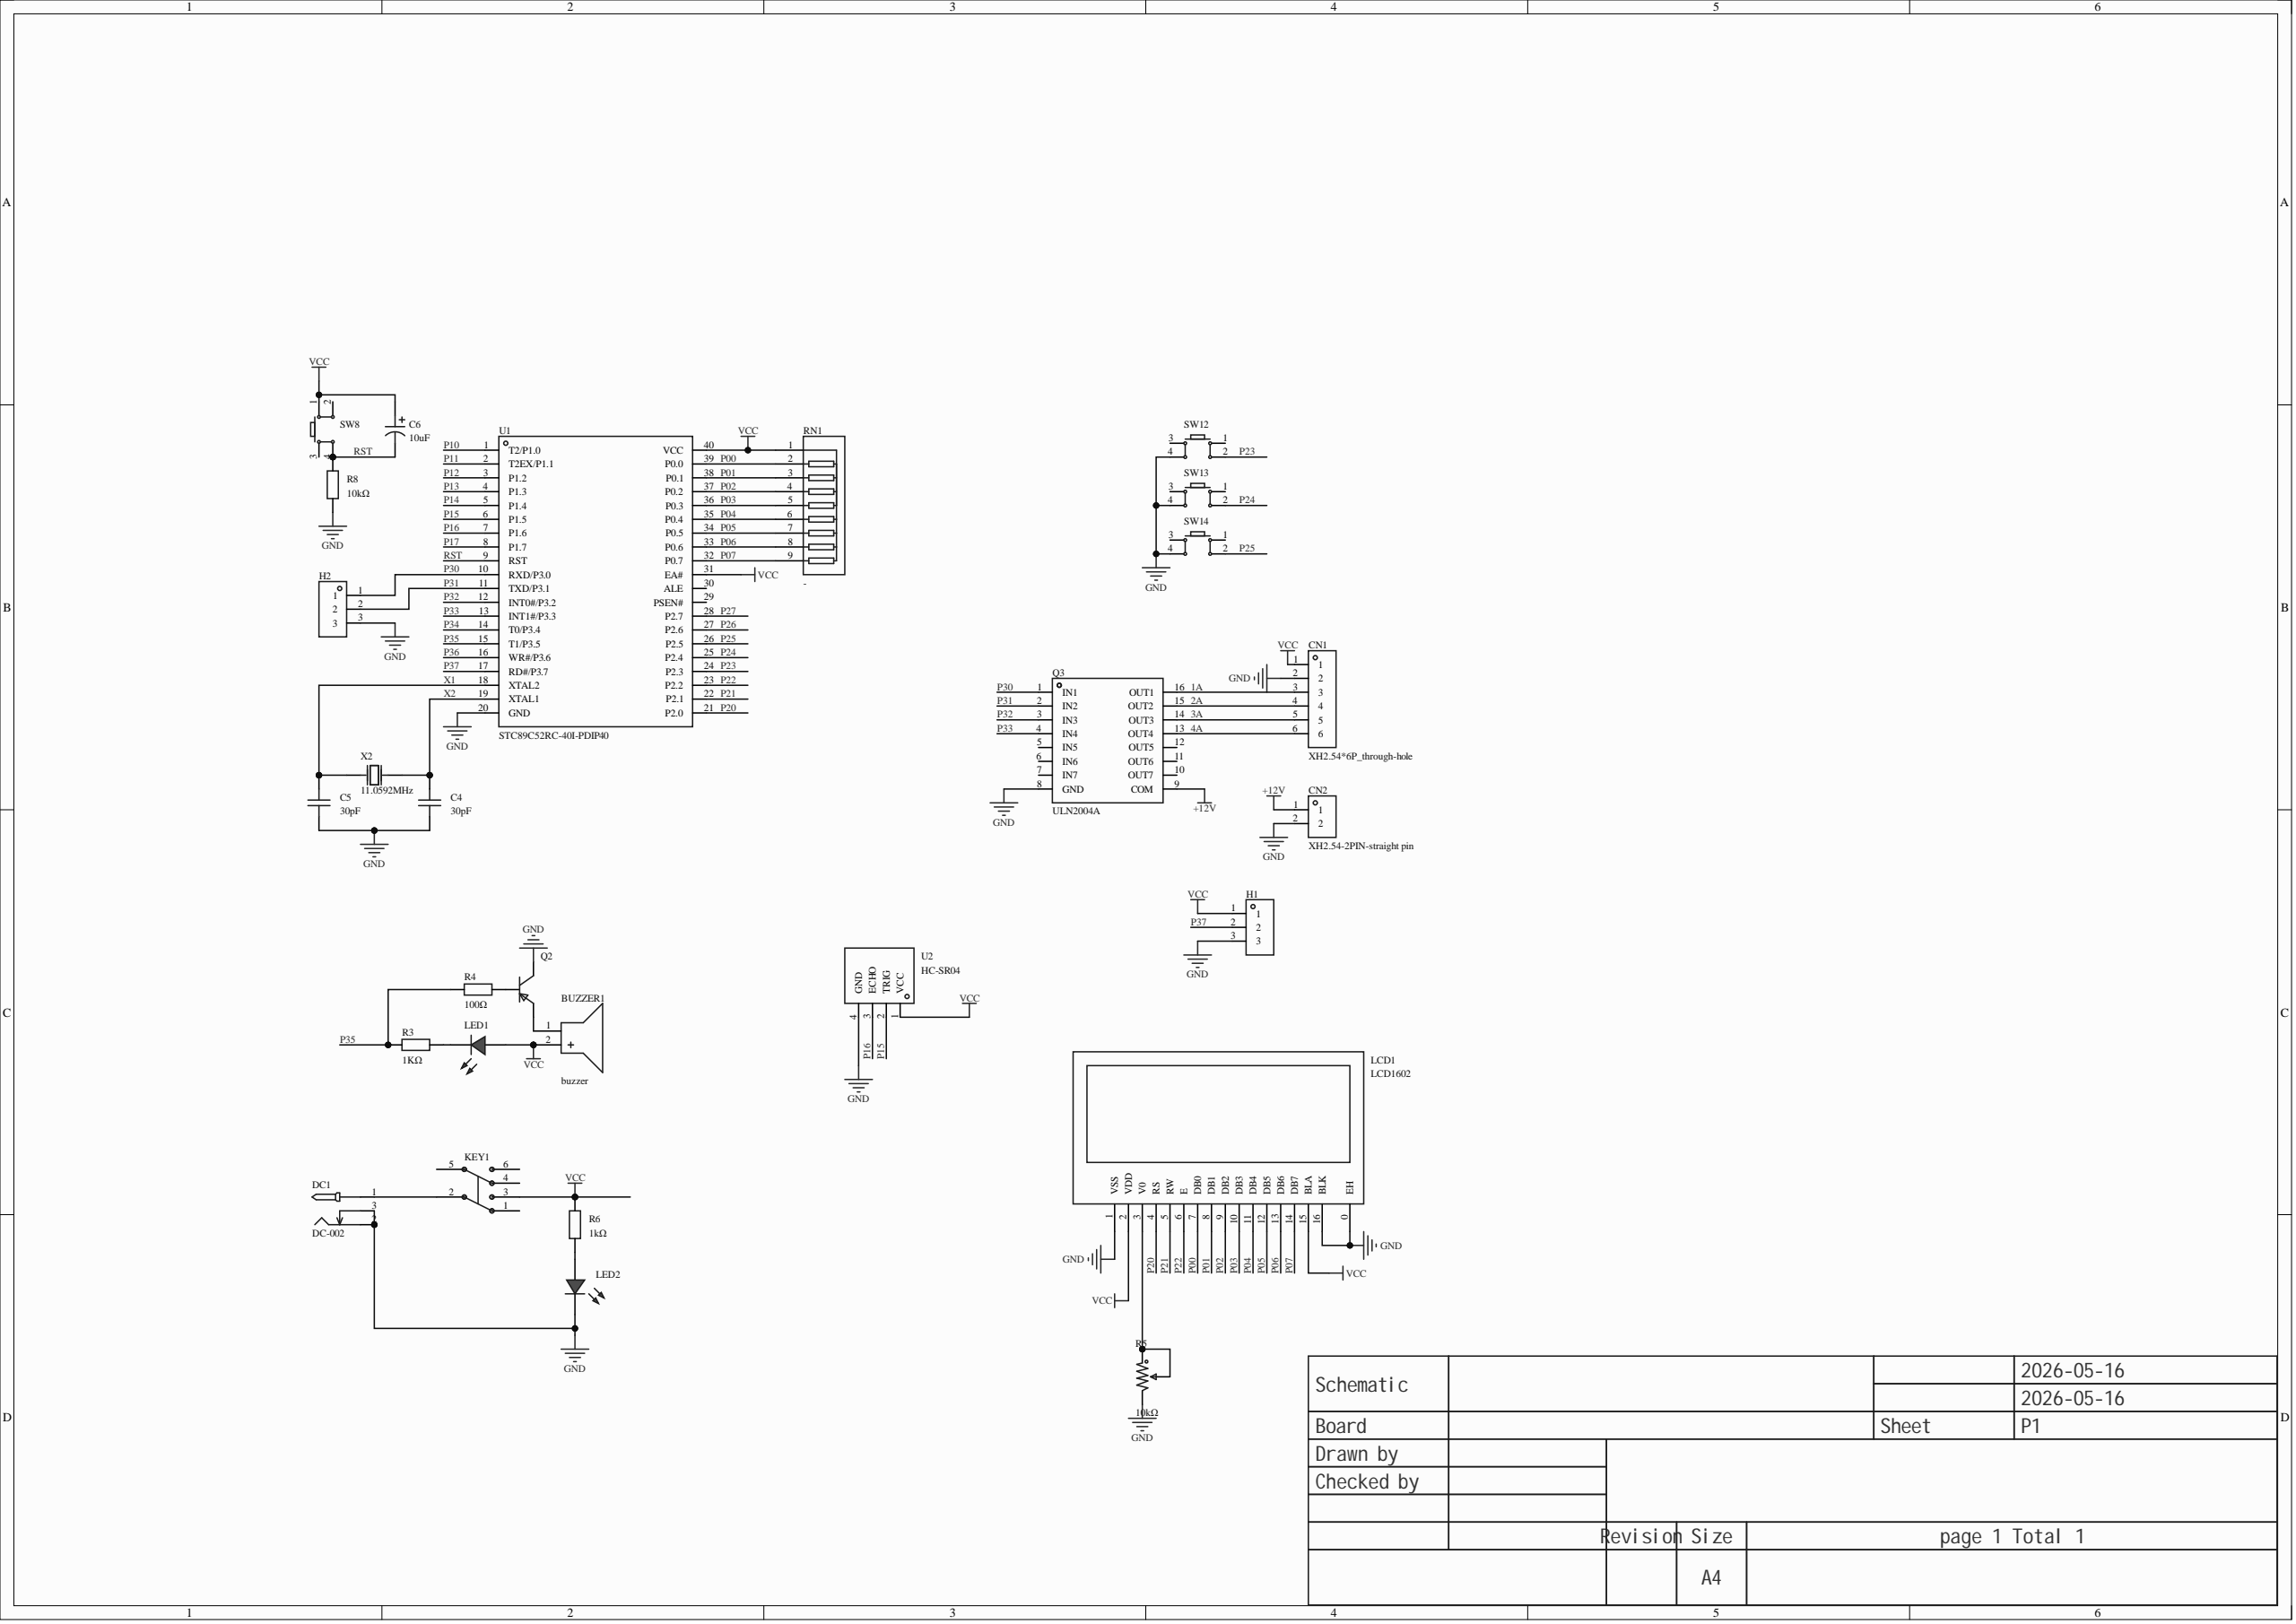Circuit board | Altium Designer | 28 parts | 38 nets
Bill of materials:
Comment,Description,Designator,Footprint,LibRef,Quantity
"buzzer","","BUZZER1","BUZ-TH_BD12.0-P6.00-D0.9-RD","buzzer","1"
"30pF","Capacitance: 30pF; tolerance: ±10%; rated voltage: 25V; temperature coefficient: C0G;","C4, C5","CAP-TH_L3.8-W2.5-P2.54-D0.50","C315C300K3G5TA7301","2"
"10uF","Capacitance: 10uF; tolerance: ±20%; rated voltage: 50V; ripple current: 120mA@100KHz; equivalent series resistance (ESR): 1.6Ω;","C6","CAP-TH_BD5.0-P2.00-D0.8-FD-10UF50VC110GL","10UF50VC110GL","1"
"XH2.54*6P_through-hole","","CN1","CONN-TH_XH2.54-6P","XH2.54*6P_直插","1"
"XH2.54-2PIN-straight pin","","CN2","CONN-TH_XH2.54-2P","XH2.54-2PIN-直针","1"
"DC-002","","DC1","DC-IN-TH_DC-3510","DC-002","1"
"","","H1","HDR-TH_3P-P2.54-V-F","HDR-F_2.54_1x3P","1"
"","","H2","HDR-TH_3P-P2.54-V-M","HDR-M_2.54_1x3P","1"
"Non-latching switch 8.5×8.5, silent","6 pins, 8.5×8.5","KEY1","SW-TH_6P-L8.5-W8.5-P2.54","无自锁开关 8.5×8.5 无声","1"
"LCD1602","Controller: SPLC780; size (inch): 2;","LCD1","LCD1602","HS1602A","1"
"","","LED1, LED2","LED_TH-3mm","LED_TH-R_3mm","2"
"","","Q2","S8550P_SOT","S8550_SOT_PNP","1"
"ULN2004A","Channels: seven; collector-emitter breakdown voltage (Vceo): 50V; collector current (Ic): 500mA;","Q3","DIP-16_L19.8-W6.5-P2.54-LS7.6-BL","ULN2004A","1"
"1KΩ","","R3, R6","Res_1/8W","Res_AXIAL-1/8W","2"
"100Ω","","R4","Res_1/8W","Res_AXIAL-1/8W","1"
"10kΩ","Resistance: 10kΩ; tolerance: ±25%; power: 100mW;","R5","RES-ADJ-SMD_RM065-V1","RM065-103(10K)","1"
"10kΩ","","R8","Res_1/8W","Res_AXIAL-1/8W","1"
"-","Number of resistors: -; resistance: -; power per element: -;","RN1","RES-ARRAY-TH_9P-P2.54-D1.0","排阻 10 K 5%","1"
"","","SW8, SW12, SW13, SW14","SW-TH_4P-L6.0-W6.0-P4.50-LS6.5","Key_TH_6x6x6","4"
"STC89C52RC-40I-PDIP40","CPU core: 51 family; CPU max frequency: -;","U1","DIP-40_L52.0-W13.7-P2.54-LS15.2-BL","STC89C52RC-40I-PDIP40","1"
"HC-SR04","","U2","TH_HC-SR04V","HC-SR04","1"
"11.059MHz","Crystal type: through-hole crystal; frequency: 11.059MHz; frequency tolerance at room temperature: ±20ppm; load capacitance: 30pF;","X2","OSC-TH_L11.1-W4.7-P4.88","9AC11059302060C3","1"
Netlist (Protel format):
[
BUZZER1
BUZ-TH_BD12.0-P6.00-D0.9-RD
buzzer



]
[
C4
CAP-TH_L3.8-W2.5-P2.54-D0.50
30pF



]
[
C5
CAP-TH_L3.8-W2.5-P2.54-D0.50
30pF



]
[
C6
CAP-TH_BD5.0-P2.00-D0.8-FD-10UF50VC110GL
10uF



]
[
CN1
CONN-TH_XH2.54-6P
XH2.54*6P_through-hole



]
[
CN2
CONN-TH_XH2.54-2P
XH2.54-2PIN-straight pin



]
[
DC1
DC-IN-TH_DC-3510
DC-002



]
[
H1
HDR-TH_3P-P2.54-V-F




]
[
H2
HDR-TH_3P-P2.54-V-M




]
[
KEY1
SW-TH_6P-L8.5-W8.5-P2.54
Non-latching switch 8.5×8.5, silent



]
[
LCD1
LCD1602
LCD1602



]
[
LED1
LED_TH-3mm




]
[
LED2
LED_TH-3mm




]
[
Q2
S8550P_SOT




]
[
Q3
DIP-16_L19.8-W6.5-P2.54-LS7.6-BL
ULN2004A



]
[
R3
Res_1/8W
1KΩ



]
[
R4
Res_1/8W
100Ω



]
[
R5
RES-ADJ-SMD_RM065-V1
10kΩ



]
[
R6
Res_1/8W
1kΩ



]
[
R8
Res_1/8W
10kΩ



]
[
RN1
RES-ARRAY-TH_9P-P2.54-D1.0
-



]
[
SW8
SW-TH_4P-L6.0-W6.0-P4.50-LS6.5




]
[
SW12
SW-TH_4P-L6.0-W6.0-P4.50-LS6.5




]
[
SW13
SW-TH_4P-L6.0-W6.0-P4.50-LS6.5




]
[
SW14
SW-TH_4P-L6.0-W6.0-P4.50-LS6.5




]
[
U1
DIP-40_L52.0-W13.7-P2.54-LS15.2-BL
STC89C52RC-40I-PDIP40



]
[
U2
TH_HC-SR04V
HC-SR04



]
[
X2
OSC-TH_L11.1-W4.7-P4.88
11.0592MHz



]
(
X2
C4-2
U1-19
X2-2
)
(
X1
C5-2
U1-18
X2-1
)
(
VCC
BUZZER1-2
C6-1
CN1-1
H1-1
KEY1-3
LCD1-2
LCD1-15
LED1-1
R6-2
RN1-1
SW8-1
U1-31
U1-40
U2-1
)
(
RST
C6-2
R8-2
SW8-4
U1-9
)
(
P37
H1-2
U1-17
)
(
P35
R3-1
R4-1
U1-15
)
(
P33
Q3-4
U1-13
)
(
P32
Q3-3
U1-12
)
(
P31
H2-2
Q3-2
U1-11
)
(
P30
H2-1
Q3-1
U1-10
)
(
P25
SW14-2
U1-26
)
(
P24
SW13-2
U1-25
)
(
P23
SW12-2
U1-24
)
(
P22
LCD1-6
U1-23
)
(
P21
LCD1-5
U1-22
)
(
P20
LCD1-4
U1-21
)
(
P16
U1-7
U2-3
)
(
P15
U1-6
U2-2
)
(
P07
LCD1-14
RN1-9
U1-32
)
(
P06
LCD1-13
RN1-8
U1-33
)
(
P05
LCD1-12
RN1-7
U1-34
)
(
P04
LCD1-11
RN1-6
U1-35
)
(
P03
LCD1-10
RN1-5
U1-36
)
(
P02
LCD1-9
RN1-4
U1-37
)
(
P01
LCD1-8
RN1-3
U1-38
)
(
P00
LCD1-7
RN1-2
U1-39
)
(
NetQ2_1
Q2-1
R4-2
)
(
NetLED2_1
LED2-1
R6-1
)
(
NetLED1_2
LED1-2
R3-2
)
(
NetLCD1_3
LCD1-3
R5-1
R5-2
)
(
NetDC1_1
DC1-1
KEY1-2
)
(
NetBUZZER1_1
BUZZER1-1
Q2-2
)
(
GND
C4-1
C5-1
CN1-2
CN2-2
DC1-2
DC1-3
H1-3
H2-3
LCD1-0
LCD1-1
LCD1-16
LED2-2
Q2-3
Q3-8
R5-3
R8-1
SW12-4
SW13-4
SW14-4
U1-20
U2-4
)
(
+12V
CN2-1
Q3-9
)
(
4A
CN1-6
Q3-13
)
(
3A
CN1-5
Q3-14
)
(
2A
CN1-4
Q3-15
)
(
1A
CN1-3
Q3-16
)